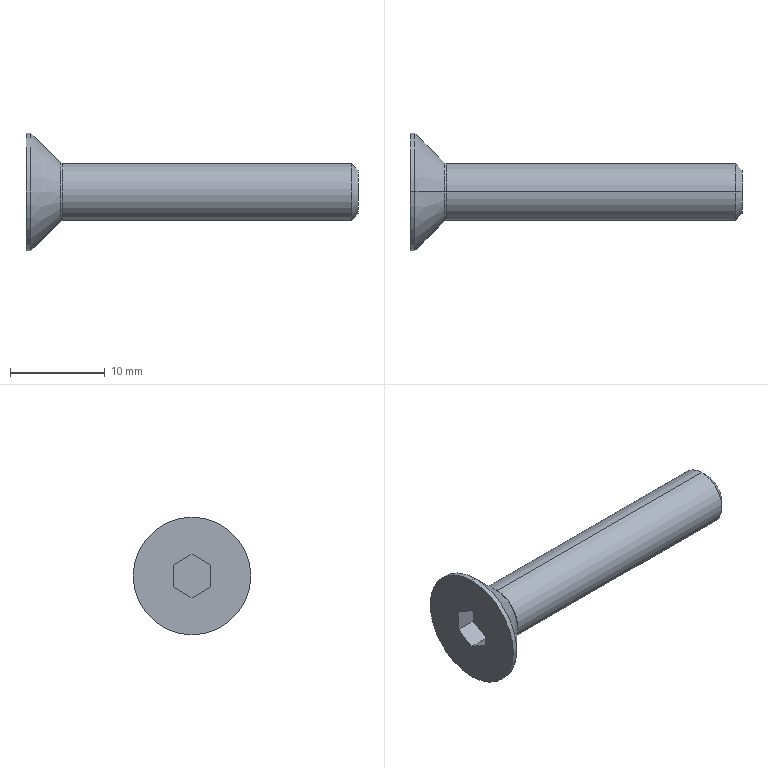Part | STEP file | 1 solid | 19 faces | box 35 x 12.399 x 12.399 mm | volume 1134 mm3 | plane 9 | cylinder 4 | cone 4 | spline 2 | commonest cylinder face diameters 6 x2 12.399 x2
STEP:
#1=CARTESIAN_POINT('',(0.,0.,0.));
#2=DIRECTION('',(0.,0.,1.));
#3=DIRECTION('',(1.,0.,0.));
#4=AXIS2_PLACEMENT_3D('',#1,#2,#3);
#5=CARTESIAN_POINT('',(-1.52,-2.,-1.155));
#6=VERTEX_POINT('',#5);
#7=CARTESIAN_POINT('',(-1.52,-2.,1.155));
#8=VERTEX_POINT('',#7);
#9=CARTESIAN_POINT('',(-1.52,-2.,-1.155));
#10=DIRECTION('',(0.,0.,1.));
#11=VECTOR('',#10,1.);
#12=LINE('',#9,#11);
#13=CARTESIAN_POINT('',(-1.52,0.,0.));
#14=DIRECTION('',(-1.,0.,0.));
#15=DIRECTION('',(0.,0.,1.));
#16=AXIS2_PLACEMENT_3D('',#13,#14,#15);
#17=PLANE('',#16);
#18=CARTESIAN_POINT('',(-1.155,-2.));
#19=DIRECTION('',(1.,0.));
#20=VECTOR('',#19,1.);
#21=LINE('',#18,#20);
#22=(GEOMETRIC_REPRESENTATION_CONTEXT(2)PARAMETRIC_REPRESENTATION_CONTEXT()REPRESENTATION_CONTEXT('',''));
#23=DEFINITIONAL_REPRESENTATION('',(#21),#22);
#24=PCURVE('',#17,#23);
#25=CARTESIAN_POINT('',(-1.52,-2.,-1.155));
#26=DIRECTION('',(0.,-1.,0.));
#27=DIRECTION('',(0.,0.,-1.));
#28=AXIS2_PLACEMENT_3D('',#25,#26,#27);
#29=PLANE('',#28);
#30=CARTESIAN_POINT('',(0.,0.));
#31=DIRECTION('',(-1.,0.));
#32=VECTOR('',#31,1.);
#33=LINE('',#30,#32);
#34=(GEOMETRIC_REPRESENTATION_CONTEXT(2)PARAMETRIC_REPRESENTATION_CONTEXT()REPRESENTATION_CONTEXT('',''));
#35=DEFINITIONAL_REPRESENTATION('',(#33),#34);
#36=PCURVE('',#29,#35);
#37=SURFACE_CURVE('',#12,(#24,#36),.PCURVE_S1.);
#38=EDGE_CURVE('',#6,#8,#37,.T.);
#39=ORIENTED_EDGE('',*,*,#38,.T.);
#40=CARTESIAN_POINT('',(-1.52,0.,2.309));
#41=VERTEX_POINT('',#40);
#42=CARTESIAN_POINT('',(-1.52,-2.,1.155));
#43=DIRECTION('',(0.,0.866,0.5));
#44=VECTOR('',#43,1.);
#45=LINE('',#42,#44);
#46=CARTESIAN_POINT('',(1.155,-2.));
#47=DIRECTION('',(0.5,0.866));
#48=VECTOR('',#47,1.);
#49=LINE('',#46,#48);
#50=(GEOMETRIC_REPRESENTATION_CONTEXT(2)PARAMETRIC_REPRESENTATION_CONTEXT()REPRESENTATION_CONTEXT('',''));
#51=DEFINITIONAL_REPRESENTATION('',(#49),#50);
#52=PCURVE('',#17,#51);
#53=CARTESIAN_POINT('',(-1.52,-2.,1.155));
#54=DIRECTION('',(0.,-0.5,0.866));
#55=DIRECTION('',(-1.,0.,0.));
#56=AXIS2_PLACEMENT_3D('',#53,#54,#55);
#57=PLANE('',#56);
#58=CARTESIAN_POINT('',(0.,0.));
#59=DIRECTION('',(0.,-1.));
#60=VECTOR('',#59,1.);
#61=LINE('',#58,#60);
#62=(GEOMETRIC_REPRESENTATION_CONTEXT(2)PARAMETRIC_REPRESENTATION_CONTEXT()REPRESENTATION_CONTEXT('',''));
#63=DEFINITIONAL_REPRESENTATION('',(#61),#62);
#64=PCURVE('',#57,#63);
#65=SURFACE_CURVE('',#45,(#52,#64),.PCURVE_S1.);
#66=EDGE_CURVE('',#8,#41,#65,.T.);
#67=ORIENTED_EDGE('',*,*,#66,.T.);
#68=CARTESIAN_POINT('',(-1.52,2.,1.155));
#69=VERTEX_POINT('',#68);
#70=CARTESIAN_POINT('',(-1.52,0.,2.309));
#71=DIRECTION('',(0.,0.866,-0.5));
#72=VECTOR('',#71,1.);
#73=LINE('',#70,#72);
#74=CARTESIAN_POINT('',(2.309,0.));
#75=DIRECTION('',(-0.5,0.866));
#76=VECTOR('',#75,1.);
#77=LINE('',#74,#76);
#78=(GEOMETRIC_REPRESENTATION_CONTEXT(2)PARAMETRIC_REPRESENTATION_CONTEXT()REPRESENTATION_CONTEXT('',''));
#79=DEFINITIONAL_REPRESENTATION('',(#77),#78);
#80=PCURVE('',#17,#79);
#81=CARTESIAN_POINT('',(-1.52,0.,2.309));
#82=DIRECTION('',(0.,0.5,0.866));
#83=DIRECTION('',(1.,0.,0.));
#84=AXIS2_PLACEMENT_3D('',#81,#82,#83);
#85=PLANE('',#84);
#86=CARTESIAN_POINT('',(0.,0.));
#87=DIRECTION('',(0.,1.));
#88=VECTOR('',#87,1.);
#89=LINE('',#86,#88);
#90=(GEOMETRIC_REPRESENTATION_CONTEXT(2)PARAMETRIC_REPRESENTATION_CONTEXT()REPRESENTATION_CONTEXT('',''));
#91=DEFINITIONAL_REPRESENTATION('',(#89),#90);
#92=PCURVE('',#85,#91);
#93=SURFACE_CURVE('',#73,(#80,#92),.PCURVE_S1.);
#94=EDGE_CURVE('',#41,#69,#93,.T.);
#95=ORIENTED_EDGE('',*,*,#94,.T.);
#96=CARTESIAN_POINT('',(-1.52,2.,-1.155));
#97=VERTEX_POINT('',#96);
#98=CARTESIAN_POINT('',(-1.52,2.,1.155));
#99=DIRECTION('',(0.,0.,-1.));
#100=VECTOR('',#99,1.);
#101=LINE('',#98,#100);
#102=CARTESIAN_POINT('',(1.155,2.));
#103=DIRECTION('',(-1.,0.));
#104=VECTOR('',#103,1.);
#105=LINE('',#102,#104);
#106=(GEOMETRIC_REPRESENTATION_CONTEXT(2)PARAMETRIC_REPRESENTATION_CONTEXT()REPRESENTATION_CONTEXT('',''));
#107=DEFINITIONAL_REPRESENTATION('',(#105),#106);
#108=PCURVE('',#17,#107);
#109=CARTESIAN_POINT('',(-1.52,2.,1.155));
#110=DIRECTION('',(0.,1.,0.));
#111=DIRECTION('',(0.,0.,-1.));
#112=AXIS2_PLACEMENT_3D('',#109,#110,#111);
#113=PLANE('',#112);
#114=CARTESIAN_POINT('',(0.,0.));
#115=DIRECTION('',(1.,0.));
#116=VECTOR('',#115,1.);
#117=LINE('',#114,#116);
#118=(GEOMETRIC_REPRESENTATION_CONTEXT(2)PARAMETRIC_REPRESENTATION_CONTEXT()REPRESENTATION_CONTEXT('',''));
#119=DEFINITIONAL_REPRESENTATION('',(#117),#118);
#120=PCURVE('',#113,#119);
#121=SURFACE_CURVE('',#101,(#108,#120),.PCURVE_S1.);
#122=EDGE_CURVE('',#69,#97,#121,.T.);
#123=ORIENTED_EDGE('',*,*,#122,.T.);
#124=CARTESIAN_POINT('',(-1.52,0.,-2.309));
#125=VERTEX_POINT('',#124);
#126=CARTESIAN_POINT('',(-1.52,2.,-1.155));
#127=DIRECTION('',(0.,-0.866,-0.5));
#128=VECTOR('',#127,1.);
#129=LINE('',#126,#128);
#130=CARTESIAN_POINT('',(-1.155,2.));
#131=DIRECTION('',(-0.5,-0.866));
#132=VECTOR('',#131,1.);
#133=LINE('',#130,#132);
#134=(GEOMETRIC_REPRESENTATION_CONTEXT(2)PARAMETRIC_REPRESENTATION_CONTEXT()REPRESENTATION_CONTEXT('',''));
#135=DEFINITIONAL_REPRESENTATION('',(#133),#134);
#136=PCURVE('',#17,#135);
#137=CARTESIAN_POINT('',(-1.52,2.,-1.155));
#138=DIRECTION('',(0.,0.5,-0.866));
#139=DIRECTION('',(-1.,0.,0.));
#140=AXIS2_PLACEMENT_3D('',#137,#138,#139);
#141=PLANE('',#140);
#142=CARTESIAN_POINT('',(0.,0.));
#143=DIRECTION('',(0.,-1.));
#144=VECTOR('',#143,1.);
#145=LINE('',#142,#144);
#146=(GEOMETRIC_REPRESENTATION_CONTEXT(2)PARAMETRIC_REPRESENTATION_CONTEXT()REPRESENTATION_CONTEXT('',''));
#147=DEFINITIONAL_REPRESENTATION('',(#145),#146);
#148=PCURVE('',#141,#147);
#149=SURFACE_CURVE('',#129,(#136,#148),.PCURVE_S1.);
#150=EDGE_CURVE('',#97,#125,#149,.T.);
#151=ORIENTED_EDGE('',*,*,#150,.T.);
#152=CARTESIAN_POINT('',(-1.52,0.,-2.309));
#153=DIRECTION('',(0.,-0.866,0.5));
#154=VECTOR('',#153,1.);
#155=LINE('',#152,#154);
#156=CARTESIAN_POINT('',(-2.309,0.));
#157=DIRECTION('',(0.5,-0.866));
#158=VECTOR('',#157,1.);
#159=LINE('',#156,#158);
#160=(GEOMETRIC_REPRESENTATION_CONTEXT(2)PARAMETRIC_REPRESENTATION_CONTEXT()REPRESENTATION_CONTEXT('',''));
#161=DEFINITIONAL_REPRESENTATION('',(#159),#160);
#162=PCURVE('',#17,#161);
#163=CARTESIAN_POINT('',(-1.52,0.,-2.309));
#164=DIRECTION('',(0.,-0.5,-0.866));
#165=DIRECTION('',(0.,-0.866,0.5));
#166=AXIS2_PLACEMENT_3D('',#163,#164,#165);
#167=PLANE('',#166);
#168=CARTESIAN_POINT('',(0.,0.));
#169=DIRECTION('',(1.,0.));
#170=VECTOR('',#169,1.);
#171=LINE('',#168,#170);
#172=(GEOMETRIC_REPRESENTATION_CONTEXT(2)PARAMETRIC_REPRESENTATION_CONTEXT()REPRESENTATION_CONTEXT('',''));
#173=DEFINITIONAL_REPRESENTATION('',(#171),#172);
#174=PCURVE('',#167,#173);
#175=SURFACE_CURVE('',#155,(#162,#174),.PCURVE_S1.);
#176=EDGE_CURVE('',#125,#6,#175,.T.);
#177=ORIENTED_EDGE('',*,*,#176,.T.);
#178=EDGE_LOOP('',(#39,#67,#95,#123,#151,#177));
#179=FACE_BOUND('',#178,.T.);
#180=ADVANCED_FACE('',(#179),#17,.T.);
#181=CARTESIAN_POINT('',(-3.72,0.,-2.309));
#182=VERTEX_POINT('',#181);
#183=CARTESIAN_POINT('',(-1.52,0.,-2.309));
#184=DIRECTION('',(1.,0.,0.));
#185=VECTOR('',#184,1.);
#186=LINE('',#183,#185);
#187=CARTESIAN_POINT('',(0.,-2.309));
#188=DIRECTION('',(-1.,0.));
#189=VECTOR('',#188,1.);
#190=LINE('',#187,#189);
#191=(GEOMETRIC_REPRESENTATION_CONTEXT(2)PARAMETRIC_REPRESENTATION_CONTEXT()REPRESENTATION_CONTEXT('',''));
#192=DEFINITIONAL_REPRESENTATION('',(#190),#191);
#193=PCURVE('',#141,#192);
#194=CARTESIAN_POINT('',(0.,0.));
#195=DIRECTION('',(0.,-1.));
#196=VECTOR('',#195,1.);
#197=LINE('',#194,#196);
#198=(GEOMETRIC_REPRESENTATION_CONTEXT(2)PARAMETRIC_REPRESENTATION_CONTEXT()REPRESENTATION_CONTEXT('',''));
#199=DEFINITIONAL_REPRESENTATION('',(#197),#198);
#200=PCURVE('',#167,#199);
#201=SURFACE_CURVE('',#186,(#193,#200),.PCURVE_S1.);
#202=EDGE_CURVE('',#182,#125,#201,.T.);
#203=ORIENTED_EDGE('',*,*,#202,.T.);
#204=ORIENTED_EDGE('',*,*,#150,.F.);
#205=CARTESIAN_POINT('',(-3.72,2.,-1.155));
#206=VERTEX_POINT('',#205);
#207=CARTESIAN_POINT('',(-1.52,2.,-1.155));
#208=DIRECTION('',(-1.,0.,0.));
#209=VECTOR('',#208,1.);
#210=LINE('',#207,#209);
#211=CARTESIAN_POINT('',(0.,0.));
#212=DIRECTION('',(1.,0.));
#213=VECTOR('',#212,1.);
#214=LINE('',#211,#213);
#215=(GEOMETRIC_REPRESENTATION_CONTEXT(2)PARAMETRIC_REPRESENTATION_CONTEXT()REPRESENTATION_CONTEXT('',''));
#216=DEFINITIONAL_REPRESENTATION('',(#214),#215);
#217=PCURVE('',#141,#216);
#218=CARTESIAN_POINT('',(2.309,0.));
#219=DIRECTION('',(0.,1.));
#220=VECTOR('',#219,1.);
#221=LINE('',#218,#220);
#222=(GEOMETRIC_REPRESENTATION_CONTEXT(2)PARAMETRIC_REPRESENTATION_CONTEXT()REPRESENTATION_CONTEXT('',''));
#223=DEFINITIONAL_REPRESENTATION('',(#221),#222);
#224=PCURVE('',#113,#223);
#225=SURFACE_CURVE('',#210,(#217,#224),.PCURVE_S1.);
#226=EDGE_CURVE('',#97,#206,#225,.T.);
#227=ORIENTED_EDGE('',*,*,#226,.T.);
#228=CARTESIAN_POINT('',(-3.72,2.,-1.155));
#229=DIRECTION('',(0.,-0.866,-0.5));
#230=VECTOR('',#229,1.);
#231=LINE('',#228,#230);
#232=CARTESIAN_POINT('',(2.2,0.));
#233=DIRECTION('',(0.,-1.));
#234=VECTOR('',#233,1.);
#235=LINE('',#232,#234);
#236=(GEOMETRIC_REPRESENTATION_CONTEXT(2)PARAMETRIC_REPRESENTATION_CONTEXT()REPRESENTATION_CONTEXT('',''));
#237=DEFINITIONAL_REPRESENTATION('',(#235),#236);
#238=PCURVE('',#141,#237);
#239=CARTESIAN_POINT('',(-3.72,6.2,0.));
#240=DIRECTION('',(1.,0.,0.));
#241=DIRECTION('',(0.,1.,0.));
#242=AXIS2_PLACEMENT_3D('',#239,#240,#241);
#243=PLANE('',#242);
#244=CARTESIAN_POINT('',(-4.2,-1.155));
#245=DIRECTION('',(-0.866,-0.5));
#246=VECTOR('',#245,1.);
#247=LINE('',#244,#246);
#248=(GEOMETRIC_REPRESENTATION_CONTEXT(2)PARAMETRIC_REPRESENTATION_CONTEXT()REPRESENTATION_CONTEXT('',''));
#249=DEFINITIONAL_REPRESENTATION('',(#247),#248);
#250=PCURVE('',#243,#249);
#251=SURFACE_CURVE('',#231,(#238,#250),.PCURVE_S1.);
#252=EDGE_CURVE('',#206,#182,#251,.T.);
#253=ORIENTED_EDGE('',*,*,#252,.T.);
#254=EDGE_LOOP('',(#203,#204,#227,#253));
#255=FACE_BOUND('',#254,.T.);
#256=ADVANCED_FACE('',(#255),#141,.F.);
#257=CARTESIAN_POINT('',(-3.72,-2.,-1.155));
#258=VERTEX_POINT('',#257);
#259=CARTESIAN_POINT('',(-1.52,-2.,-1.155));
#260=DIRECTION('',(1.,0.,0.));
#261=VECTOR('',#260,1.);
#262=LINE('',#259,#261);
#263=CARTESIAN_POINT('',(2.309,0.));
#264=DIRECTION('',(0.,-1.));
#265=VECTOR('',#264,1.);
#266=LINE('',#263,#265);
#267=(GEOMETRIC_REPRESENTATION_CONTEXT(2)PARAMETRIC_REPRESENTATION_CONTEXT()REPRESENTATION_CONTEXT('',''));
#268=DEFINITIONAL_REPRESENTATION('',(#266),#267);
#269=PCURVE('',#167,#268);
#270=CARTESIAN_POINT('',(0.,0.));
#271=DIRECTION('',(0.,1.));
#272=VECTOR('',#271,1.);
#273=LINE('',#270,#272);
#274=(GEOMETRIC_REPRESENTATION_CONTEXT(2)PARAMETRIC_REPRESENTATION_CONTEXT()REPRESENTATION_CONTEXT('',''));
#275=DEFINITIONAL_REPRESENTATION('',(#273),#274);
#276=PCURVE('',#29,#275);
#277=SURFACE_CURVE('',#262,(#269,#276),.PCURVE_S1.);
#278=EDGE_CURVE('',#258,#6,#277,.T.);
#279=ORIENTED_EDGE('',*,*,#278,.T.);
#280=ORIENTED_EDGE('',*,*,#176,.F.);
#281=ORIENTED_EDGE('',*,*,#202,.F.);
#282=CARTESIAN_POINT('',(-3.72,0.,-2.309));
#283=DIRECTION('',(0.,-0.866,0.5));
#284=VECTOR('',#283,1.);
#285=LINE('',#282,#284);
#286=CARTESIAN_POINT('',(0.,2.2));
#287=DIRECTION('',(1.,0.));
#288=VECTOR('',#287,1.);
#289=LINE('',#286,#288);
#290=(GEOMETRIC_REPRESENTATION_CONTEXT(2)PARAMETRIC_REPRESENTATION_CONTEXT()REPRESENTATION_CONTEXT('',''));
#291=DEFINITIONAL_REPRESENTATION('',(#289),#290);
#292=PCURVE('',#167,#291);
#293=CARTESIAN_POINT('',(-6.2,-2.309));
#294=DIRECTION('',(-0.866,0.5));
#295=VECTOR('',#294,1.);
#296=LINE('',#293,#295);
#297=(GEOMETRIC_REPRESENTATION_CONTEXT(2)PARAMETRIC_REPRESENTATION_CONTEXT()REPRESENTATION_CONTEXT('',''));
#298=DEFINITIONAL_REPRESENTATION('',(#296),#297);
#299=PCURVE('',#243,#298);
#300=SURFACE_CURVE('',#285,(#292,#299),.PCURVE_S1.);
#301=EDGE_CURVE('',#182,#258,#300,.T.);
#302=ORIENTED_EDGE('',*,*,#301,.T.);
#303=EDGE_LOOP('',(#279,#280,#281,#302));
#304=FACE_BOUND('',#303,.T.);
#305=ADVANCED_FACE('',(#304),#167,.F.);
#306=CARTESIAN_POINT('',(-3.72,-2.,1.155));
#307=VERTEX_POINT('',#306);
#308=CARTESIAN_POINT('',(-1.52,-2.,1.155));
#309=DIRECTION('',(1.,0.,0.));
#310=VECTOR('',#309,1.);
#311=LINE('',#308,#310);
#312=CARTESIAN_POINT('',(-2.309,0.));
#313=DIRECTION('',(0.,1.));
#314=VECTOR('',#313,1.);
#315=LINE('',#312,#314);
#316=(GEOMETRIC_REPRESENTATION_CONTEXT(2)PARAMETRIC_REPRESENTATION_CONTEXT()REPRESENTATION_CONTEXT('',''));
#317=DEFINITIONAL_REPRESENTATION('',(#315),#316);
#318=PCURVE('',#29,#317);
#319=CARTESIAN_POINT('',(0.,0.));
#320=DIRECTION('',(-1.,0.));
#321=VECTOR('',#320,1.);
#322=LINE('',#319,#321);
#323=(GEOMETRIC_REPRESENTATION_CONTEXT(2)PARAMETRIC_REPRESENTATION_CONTEXT()REPRESENTATION_CONTEXT('',''));
#324=DEFINITIONAL_REPRESENTATION('',(#322),#323);
#325=PCURVE('',#57,#324);
#326=SURFACE_CURVE('',#311,(#318,#325),.PCURVE_S1.);
#327=EDGE_CURVE('',#307,#8,#326,.T.);
#328=ORIENTED_EDGE('',*,*,#327,.T.);
#329=ORIENTED_EDGE('',*,*,#38,.F.);
#330=ORIENTED_EDGE('',*,*,#278,.F.);
#331=CARTESIAN_POINT('',(-3.72,-2.,0.));
#332=DIRECTION('',(0.,0.,1.));
#333=VECTOR('',#332,1.);
#334=LINE('',#331,#333);
#335=CARTESIAN_POINT('',(-1.155,-2.2));
#336=DIRECTION('',(-1.,0.));
#337=VECTOR('',#336,1.);
#338=LINE('',#335,#337);
#339=(GEOMETRIC_REPRESENTATION_CONTEXT(2)PARAMETRIC_REPRESENTATION_CONTEXT()REPRESENTATION_CONTEXT('',''));
#340=DEFINITIONAL_REPRESENTATION('',(#338),#339);
#341=PCURVE('',#29,#340);
#342=CARTESIAN_POINT('',(-8.2,0.));
#343=DIRECTION('',(0.,1.));
#344=VECTOR('',#343,1.);
#345=LINE('',#342,#344);
#346=(GEOMETRIC_REPRESENTATION_CONTEXT(2)PARAMETRIC_REPRESENTATION_CONTEXT()REPRESENTATION_CONTEXT('',''));
#347=DEFINITIONAL_REPRESENTATION('',(#345),#346);
#348=PCURVE('',#243,#347);
#349=SURFACE_CURVE('',#334,(#341,#348),.PCURVE_S1.);
#350=EDGE_CURVE('',#258,#307,#349,.T.);
#351=ORIENTED_EDGE('',*,*,#350,.T.);
#352=EDGE_LOOP('',(#328,#329,#330,#351));
#353=FACE_BOUND('',#352,.T.);
#354=ADVANCED_FACE('',(#353),#29,.F.);
#355=CARTESIAN_POINT('',(-3.72,0.,2.309));
#356=VERTEX_POINT('',#355);
#357=CARTESIAN_POINT('',(-1.52,0.,2.309));
#358=DIRECTION('',(1.,0.,0.));
#359=VECTOR('',#358,1.);
#360=LINE('',#357,#359);
#361=CARTESIAN_POINT('',(0.,-2.309));
#362=DIRECTION('',(-1.,0.));
#363=VECTOR('',#362,1.);
#364=LINE('',#361,#363);
#365=(GEOMETRIC_REPRESENTATION_CONTEXT(2)PARAMETRIC_REPRESENTATION_CONTEXT()REPRESENTATION_CONTEXT('',''));
#366=DEFINITIONAL_REPRESENTATION('',(#364),#365);
#367=PCURVE('',#57,#366);
#368=CARTESIAN_POINT('',(0.,0.));
#369=DIRECTION('',(1.,0.));
#370=VECTOR('',#369,1.);
#371=LINE('',#368,#370);
#372=(GEOMETRIC_REPRESENTATION_CONTEXT(2)PARAMETRIC_REPRESENTATION_CONTEXT()REPRESENTATION_CONTEXT('',''));
#373=DEFINITIONAL_REPRESENTATION('',(#371),#372);
#374=PCURVE('',#85,#373);
#375=SURFACE_CURVE('',#360,(#367,#374),.PCURVE_S1.);
#376=EDGE_CURVE('',#356,#41,#375,.T.);
#377=ORIENTED_EDGE('',*,*,#376,.T.);
#378=ORIENTED_EDGE('',*,*,#66,.F.);
#379=ORIENTED_EDGE('',*,*,#327,.F.);
#380=CARTESIAN_POINT('',(-3.72,-2.,1.155));
#381=DIRECTION('',(0.,0.866,0.5));
#382=VECTOR('',#381,1.);
#383=LINE('',#380,#382);
#384=CARTESIAN_POINT('',(2.2,0.));
#385=DIRECTION('',(0.,-1.));
#386=VECTOR('',#385,1.);
#387=LINE('',#384,#386);
#388=(GEOMETRIC_REPRESENTATION_CONTEXT(2)PARAMETRIC_REPRESENTATION_CONTEXT()REPRESENTATION_CONTEXT('',''));
#389=DEFINITIONAL_REPRESENTATION('',(#387),#388);
#390=PCURVE('',#57,#389);
#391=CARTESIAN_POINT('',(-8.2,1.155));
#392=DIRECTION('',(0.866,0.5));
#393=VECTOR('',#392,1.);
#394=LINE('',#391,#393);
#395=(GEOMETRIC_REPRESENTATION_CONTEXT(2)PARAMETRIC_REPRESENTATION_CONTEXT()REPRESENTATION_CONTEXT('',''));
#396=DEFINITIONAL_REPRESENTATION('',(#394),#395);
#397=PCURVE('',#243,#396);
#398=SURFACE_CURVE('',#383,(#390,#397),.PCURVE_S1.);
#399=EDGE_CURVE('',#307,#356,#398,.T.);
#400=ORIENTED_EDGE('',*,*,#399,.T.);
#401=EDGE_LOOP('',(#377,#378,#379,#400));
#402=FACE_BOUND('',#401,.T.);
#403=ADVANCED_FACE('',(#402),#57,.F.);
#404=CARTESIAN_POINT('',(-3.72,2.,1.155));
#405=VERTEX_POINT('',#404);
#406=CARTESIAN_POINT('',(-1.52,2.,1.155));
#407=DIRECTION('',(1.,0.,0.));
#408=VECTOR('',#407,1.);
#409=LINE('',#406,#408);
#410=CARTESIAN_POINT('',(0.,2.309));
#411=DIRECTION('',(1.,0.));
#412=VECTOR('',#411,1.);
#413=LINE('',#410,#412);
#414=(GEOMETRIC_REPRESENTATION_CONTEXT(2)PARAMETRIC_REPRESENTATION_CONTEXT()REPRESENTATION_CONTEXT('',''));
#415=DEFINITIONAL_REPRESENTATION('',(#413),#414);
#416=PCURVE('',#85,#415);
#417=CARTESIAN_POINT('',(0.,0.));
#418=DIRECTION('',(0.,-1.));
#419=VECTOR('',#418,1.);
#420=LINE('',#417,#419);
#421=(GEOMETRIC_REPRESENTATION_CONTEXT(2)PARAMETRIC_REPRESENTATION_CONTEXT()REPRESENTATION_CONTEXT('',''));
#422=DEFINITIONAL_REPRESENTATION('',(#420),#421);
#423=PCURVE('',#113,#422);
#424=SURFACE_CURVE('',#409,(#416,#423),.PCURVE_S1.);
#425=EDGE_CURVE('',#405,#69,#424,.T.);
#426=ORIENTED_EDGE('',*,*,#425,.T.);
#427=ORIENTED_EDGE('',*,*,#94,.F.);
#428=ORIENTED_EDGE('',*,*,#376,.F.);
#429=CARTESIAN_POINT('',(-3.72,0.,2.309));
#430=DIRECTION('',(0.,0.866,-0.5));
#431=VECTOR('',#430,1.);
#432=LINE('',#429,#431);
#433=CARTESIAN_POINT('',(-2.2,0.));
#434=DIRECTION('',(0.,1.));
#435=VECTOR('',#434,1.);
#436=LINE('',#433,#435);
#437=(GEOMETRIC_REPRESENTATION_CONTEXT(2)PARAMETRIC_REPRESENTATION_CONTEXT()REPRESENTATION_CONTEXT('',''));
#438=DEFINITIONAL_REPRESENTATION('',(#436),#437);
#439=PCURVE('',#85,#438);
#440=CARTESIAN_POINT('',(-6.2,2.309));
#441=DIRECTION('',(0.866,-0.5));
#442=VECTOR('',#441,1.);
#443=LINE('',#440,#442);
#444=(GEOMETRIC_REPRESENTATION_CONTEXT(2)PARAMETRIC_REPRESENTATION_CONTEXT()REPRESENTATION_CONTEXT('',''));
#445=DEFINITIONAL_REPRESENTATION('',(#443),#444);
#446=PCURVE('',#243,#445);
#447=SURFACE_CURVE('',#432,(#439,#446),.PCURVE_S1.);
#448=EDGE_CURVE('',#356,#405,#447,.T.);
#449=ORIENTED_EDGE('',*,*,#448,.T.);
#450=EDGE_LOOP('',(#426,#427,#428,#449));
#451=FACE_BOUND('',#450,.T.);
#452=ADVANCED_FACE('',(#451),#85,.F.);
#453=ORIENTED_EDGE('',*,*,#226,.F.);
#454=ORIENTED_EDGE('',*,*,#122,.F.);
#455=ORIENTED_EDGE('',*,*,#425,.F.);
#456=CARTESIAN_POINT('',(-3.72,2.,0.));
#457=DIRECTION('',(0.,0.,-1.));
#458=VECTOR('',#457,1.);
#459=LINE('',#456,#458);
#460=CARTESIAN_POINT('',(1.155,2.2));
#461=DIRECTION('',(1.,0.));
#462=VECTOR('',#461,1.);
#463=LINE('',#460,#462);
#464=(GEOMETRIC_REPRESENTATION_CONTEXT(2)PARAMETRIC_REPRESENTATION_CONTEXT()REPRESENTATION_CONTEXT('',''));
#465=DEFINITIONAL_REPRESENTATION('',(#463),#464);
#466=PCURVE('',#113,#465);
#467=CARTESIAN_POINT('',(-4.2,0.));
#468=DIRECTION('',(0.,-1.));
#469=VECTOR('',#468,1.);
#470=LINE('',#467,#469);
#471=(GEOMETRIC_REPRESENTATION_CONTEXT(2)PARAMETRIC_REPRESENTATION_CONTEXT()REPRESENTATION_CONTEXT('',''));
#472=DEFINITIONAL_REPRESENTATION('',(#470),#471);
#473=PCURVE('',#243,#472);
#474=SURFACE_CURVE('',#459,(#466,#473),.PCURVE_S1.);
#475=EDGE_CURVE('',#405,#206,#474,.T.);
#476=ORIENTED_EDGE('',*,*,#475,.T.);
#477=EDGE_LOOP('',(#453,#454,#455,#476));
#478=FACE_BOUND('',#477,.T.);
#479=ADVANCED_FACE('',(#478),#113,.F.);
#480=ORIENTED_EDGE('',*,*,#448,.F.);
#481=ORIENTED_EDGE('',*,*,#399,.F.);
#482=ORIENTED_EDGE('',*,*,#350,.F.);
#483=ORIENTED_EDGE('',*,*,#301,.F.);
#484=ORIENTED_EDGE('',*,*,#252,.F.);
#485=ORIENTED_EDGE('',*,*,#475,.F.);
#486=EDGE_LOOP('',(#480,#481,#482,#483,#484,#485));
#487=FACE_BOUND('',#486,.T.);
#488=CARTESIAN_POINT('',(-3.72,0.,6.2));
#489=VERTEX_POINT('',#488);
#490=CARTESIAN_POINT('',(-3.72,0.,-6.2));
#491=VERTEX_POINT('',#490);
#492=CARTESIAN_POINT('',(-3.72,0.,0.));
#493=DIRECTION('',(1.,0.,0.));
#494=DIRECTION('',(0.,0.,1.));
#495=AXIS2_PLACEMENT_3D('',#492,#493,#494);
#496=CIRCLE('',#495,6.2);
#497=CARTESIAN_POINT('',(-6.2,0.));
#498=DIRECTION('',(0.,1.));
#499=AXIS2_PLACEMENT_2D('',#497,#498);
#500=CIRCLE('',#499,6.2);
#501=(GEOMETRIC_REPRESENTATION_CONTEXT(2)PARAMETRIC_REPRESENTATION_CONTEXT()REPRESENTATION_CONTEXT('',''));
#502=DEFINITIONAL_REPRESENTATION('',(#500),#501);
#503=PCURVE('',#243,#502);
#504=CARTESIAN_POINT('',(-30.898,0.,0.));
#505=DIRECTION('',(-1.,0.,0.));
#506=DIRECTION('',(0.,0.,1.));
#507=AXIS2_PLACEMENT_3D('',#504,#505,#506);
#508=CYLINDRICAL_SURFACE('',#507,6.2);
#509=CARTESIAN_POINT('',(6.283,-27.178));
#510=DIRECTION('',(-1.,0.));
#511=VECTOR('',#510,1.);
#512=LINE('',#509,#511);
#513=(GEOMETRIC_REPRESENTATION_CONTEXT(2)PARAMETRIC_REPRESENTATION_CONTEXT()REPRESENTATION_CONTEXT('',''));
#514=DEFINITIONAL_REPRESENTATION('',(#512),#513);
#515=PCURVE('',#508,#514);
#516=SURFACE_CURVE('',#496,(#503,#515),.PCURVE_S1.);
#517=EDGE_CURVE('',#489,#491,#516,.T.);
#518=ORIENTED_EDGE('',*,*,#517,.F.);
#519=CARTESIAN_POINT('',(-3.72,0.,0.));
#520=DIRECTION('',(1.,0.,0.));
#521=DIRECTION('',(0.,0.,1.));
#522=AXIS2_PLACEMENT_3D('',#519,#520,#521);
#523=CIRCLE('',#522,6.2);
#524=CARTESIAN_POINT('',(-6.2,0.));
#525=DIRECTION('',(0.,1.));
#526=AXIS2_PLACEMENT_2D('',#524,#525);
#527=CIRCLE('',#526,6.2);
#528=(GEOMETRIC_REPRESENTATION_CONTEXT(2)PARAMETRIC_REPRESENTATION_CONTEXT()REPRESENTATION_CONTEXT('',''));
#529=DEFINITIONAL_REPRESENTATION('',(#527),#528);
#530=PCURVE('',#243,#529);
#531=CARTESIAN_POINT('',(-30.898,0.,0.));
#532=DIRECTION('',(-1.,0.,0.));
#533=DIRECTION('',(0.,0.,1.));
#534=AXIS2_PLACEMENT_3D('',#531,#532,#533);
#535=CYLINDRICAL_SURFACE('',#534,6.2);
#536=CARTESIAN_POINT('',(6.283,-27.178));
#537=DIRECTION('',(-1.,0.));
#538=VECTOR('',#537,1.);
#539=LINE('',#536,#538);
#540=(GEOMETRIC_REPRESENTATION_CONTEXT(2)PARAMETRIC_REPRESENTATION_CONTEXT()REPRESENTATION_CONTEXT('',''));
#541=DEFINITIONAL_REPRESENTATION('',(#539),#540);
#542=PCURVE('',#535,#541);
#543=SURFACE_CURVE('',#523,(#530,#542),.PCURVE_S1.);
#544=EDGE_CURVE('',#491,#489,#543,.T.);
#545=ORIENTED_EDGE('',*,*,#544,.F.);
#546=EDGE_LOOP('',(#518,#545));
#547=FACE_BOUND('',#546,.T.);
#548=ADVANCED_FACE('',(#487,#547),#243,.F.);
#549=CARTESIAN_POINT('',(-3.2,0.,-6.2));
#550=VERTEX_POINT('',#549);
#551=CARTESIAN_POINT('',(-30.898,0.,-6.2));
#552=DIRECTION('',(-1.,0.,0.));
#553=VECTOR('',#552,1.);
#554=LINE('',#551,#553);
#555=CARTESIAN_POINT('',(3.142,0.));
#556=DIRECTION('',(0.,1.));
#557=VECTOR('',#556,1.);
#558=LINE('',#555,#557);
#559=(GEOMETRIC_REPRESENTATION_CONTEXT(2)PARAMETRIC_REPRESENTATION_CONTEXT()REPRESENTATION_CONTEXT('',''));
#560=DEFINITIONAL_REPRESENTATION('',(#558),#559);
#561=PCURVE('',#508,#560);
#562=CARTESIAN_POINT('',(3.142,0.));
#563=DIRECTION('',(0.,1.));
#564=VECTOR('',#563,1.);
#565=LINE('',#562,#564);
#566=(GEOMETRIC_REPRESENTATION_CONTEXT(2)PARAMETRIC_REPRESENTATION_CONTEXT()REPRESENTATION_CONTEXT('',''));
#567=DEFINITIONAL_REPRESENTATION('',(#565),#566);
#568=PCURVE('',#535,#567);
#569=SURFACE_CURVE('',#554,(#561,#568),.PCURVE_S1.);
#570=EDGE_CURVE('',#550,#491,#569,.T.);
#571=ORIENTED_EDGE('',*,*,#570,.F.);
#572=CARTESIAN_POINT('',(-3.2,0.,6.2));
#573=VERTEX_POINT('',#572);
#574=CARTESIAN_POINT('',(-3.2,0.,0.));
#575=DIRECTION('',(1.,0.,0.));
#576=DIRECTION('',(0.,0.,1.));
#577=AXIS2_PLACEMENT_3D('',#574,#575,#576);
#578=CIRCLE('',#577,6.2);
#579=CARTESIAN_POINT('',(6.283,-27.698));
#580=DIRECTION('',(-1.,0.));
#581=VECTOR('',#580,1.);
#582=LINE('',#579,#581);
#583=(GEOMETRIC_REPRESENTATION_CONTEXT(2)PARAMETRIC_REPRESENTATION_CONTEXT()REPRESENTATION_CONTEXT('',''));
#584=DEFINITIONAL_REPRESENTATION('',(#582),#583);
#585=PCURVE('',#508,#584);
#586=CARTESIAN_POINT('',(-3.2,0.,0.));
#587=DIRECTION('',(-1.,0.,0.));
#588=DIRECTION('',(0.,0.,1.));
#589=AXIS2_PLACEMENT_3D('',#586,#587,#588);
#590=CONICAL_SURFACE('',#589,6.2,0.7854);
#591=CARTESIAN_POINT('',(6.283,0.));
#592=DIRECTION('',(-1.,0.));
#593=VECTOR('',#592,1.);
#594=LINE('',#591,#593);
#595=(GEOMETRIC_REPRESENTATION_CONTEXT(2)PARAMETRIC_REPRESENTATION_CONTEXT()REPRESENTATION_CONTEXT('',''));
#596=DEFINITIONAL_REPRESENTATION('',(#594),#595);
#597=PCURVE('',#590,#596);
#598=SURFACE_CURVE('',#578,(#585,#597),.PCURVE_S1.);
#599=EDGE_CURVE('',#573,#550,#598,.T.);
#600=ORIENTED_EDGE('',*,*,#599,.F.);
#601=CARTESIAN_POINT('',(-30.898,0.,6.2));
#602=DIRECTION('',(-1.,0.,0.));
#603=VECTOR('',#602,1.);
#604=LINE('',#601,#603);
#605=CARTESIAN_POINT('',(6.283,0.));
#606=DIRECTION('',(0.,1.));
#607=VECTOR('',#606,1.);
#608=LINE('',#605,#607);
#609=(GEOMETRIC_REPRESENTATION_CONTEXT(2)PARAMETRIC_REPRESENTATION_CONTEXT()REPRESENTATION_CONTEXT('',''));
#610=DEFINITIONAL_REPRESENTATION('',(#608),#609);
#611=PCURVE('',#508,#610);
#612=CARTESIAN_POINT('',(0.,0.));
#613=DIRECTION('',(0.,1.));
#614=VECTOR('',#613,1.);
#615=LINE('',#612,#614);
#616=(GEOMETRIC_REPRESENTATION_CONTEXT(2)PARAMETRIC_REPRESENTATION_CONTEXT()REPRESENTATION_CONTEXT('',''));
#617=DEFINITIONAL_REPRESENTATION('',(#615),#616);
#618=PCURVE('',#535,#617);
#619=SURFACE_CURVE('',#604,(#611,#618),.PCURVE_S1.);
#620=EDGE_CURVE('',#573,#489,#619,.T.);
#621=ORIENTED_EDGE('',*,*,#620,.T.);
#622=ORIENTED_EDGE('',*,*,#517,.T.);
#623=EDGE_LOOP('',(#571,#600,#621,#622));
#624=FACE_BOUND('',#623,.T.);
#625=ADVANCED_FACE('',(#624),#508,.T.);
#626=CARTESIAN_POINT('',(31.28,0.,2.3));
#627=VERTEX_POINT('',#626);
#628=CARTESIAN_POINT('',(31.28,0.,-2.3));
#629=VERTEX_POINT('',#628);
#630=CARTESIAN_POINT('',(31.28,0.,0.));
#631=DIRECTION('',(-1.,0.,0.));
#632=DIRECTION('',(0.,0.,1.));
#633=AXIS2_PLACEMENT_3D('',#630,#631,#632);
#634=CIRCLE('',#633,2.3);
#635=CARTESIAN_POINT('',(31.28,3.,0.));
#636=DIRECTION('',(-1.,0.,0.));
#637=DIRECTION('',(0.,0.,1.));
#638=AXIS2_PLACEMENT_3D('',#635,#636,#637);
#639=PLANE('',#638);
#640=CARTESIAN_POINT('',(0.,-3.));
#641=DIRECTION('',(1.,0.));
#642=AXIS2_PLACEMENT_2D('',#640,#641);
#643=CIRCLE('',#642,2.3);
#644=(GEOMETRIC_REPRESENTATION_CONTEXT(2)PARAMETRIC_REPRESENTATION_CONTEXT()REPRESENTATION_CONTEXT('',''));
#645=DEFINITIONAL_REPRESENTATION('',(#643),#644);
#646=PCURVE('',#639,#645);
#647=CARTESIAN_POINT('',(30.58,0.,0.));
#648=DIRECTION('',(-1.,0.,0.));
#649=DIRECTION('',(0.,0.,1.));
#650=AXIS2_PLACEMENT_3D('',#647,#648,#649);
#651=CONICAL_SURFACE('',#650,3.,0.7854);
#652=CARTESIAN_POINT('',(0.,-0.7));
#653=DIRECTION('',(1.,0.));
#654=VECTOR('',#653,1.);
#655=LINE('',#652,#654);
#656=(GEOMETRIC_REPRESENTATION_CONTEXT(2)PARAMETRIC_REPRESENTATION_CONTEXT()REPRESENTATION_CONTEXT('',''));
#657=DEFINITIONAL_REPRESENTATION('',(#655),#656);
#658=PCURVE('',#651,#657);
#659=SURFACE_CURVE('',#634,(#646,#658),.PCURVE_S1.);
#660=EDGE_CURVE('',#627,#629,#659,.T.);
#661=ORIENTED_EDGE('',*,*,#660,.F.);
#662=CARTESIAN_POINT('',(31.28,0.,0.));
#663=DIRECTION('',(-1.,0.,0.));
#664=DIRECTION('',(0.,0.,1.));
#665=AXIS2_PLACEMENT_3D('',#662,#663,#664);
#666=CIRCLE('',#665,2.3);
#667=CARTESIAN_POINT('',(0.,-3.));
#668=DIRECTION('',(1.,0.));
#669=AXIS2_PLACEMENT_2D('',#667,#668);
#670=CIRCLE('',#669,2.3);
#671=(GEOMETRIC_REPRESENTATION_CONTEXT(2)PARAMETRIC_REPRESENTATION_CONTEXT()REPRESENTATION_CONTEXT('',''));
#672=DEFINITIONAL_REPRESENTATION('',(#670),#671);
#673=PCURVE('',#639,#672);
#674=CARTESIAN_POINT('',(30.58,0.,0.));
#675=DIRECTION('',(-1.,0.,0.));
#676=DIRECTION('',(0.,0.,1.));
#677=AXIS2_PLACEMENT_3D('',#674,#675,#676);
#678=CONICAL_SURFACE('',#677,3.,0.7854);
#679=CARTESIAN_POINT('',(0.,-0.7));
#680=DIRECTION('',(1.,0.));
#681=VECTOR('',#680,1.);
#682=LINE('',#679,#681);
#683=(GEOMETRIC_REPRESENTATION_CONTEXT(2)PARAMETRIC_REPRESENTATION_CONTEXT()REPRESENTATION_CONTEXT('',''));
#684=DEFINITIONAL_REPRESENTATION('',(#682),#683);
#685=PCURVE('',#678,#684);
#686=SURFACE_CURVE('',#666,(#673,#685),.PCURVE_S1.);
#687=EDGE_CURVE('',#629,#627,#686,.T.);
#688=ORIENTED_EDGE('',*,*,#687,.F.);
#689=EDGE_LOOP('',(#661,#688));
#690=FACE_BOUND('',#689,.T.);
#691=ADVANCED_FACE('',(#690),#639,.F.);
#692=CARTESIAN_POINT('',(-0.07322,0.,-3.073));
#693=VERTEX_POINT('',#692);
#694=CARTESIAN_POINT('',(-3.2,0.,-6.2));
#695=DIRECTION('',(-0.7071,0.,-0.7071));
#696=VECTOR('',#695,1.);
#697=LINE('',#694,#696);
#698=CARTESIAN_POINT('',(3.142,0.));
#699=DIRECTION('',(0.,1.));
#700=VECTOR('',#699,1.);
#701=LINE('',#698,#700);
#702=(GEOMETRIC_REPRESENTATION_CONTEXT(2)PARAMETRIC_REPRESENTATION_CONTEXT()REPRESENTATION_CONTEXT('',''));
#703=DEFINITIONAL_REPRESENTATION('',(#701),#702);
#704=PCURVE('',#590,#703);
#705=CARTESIAN_POINT('',(-3.2,0.,0.));
#706=DIRECTION('',(-1.,0.,0.));
#707=DIRECTION('',(0.,0.,1.));
#708=AXIS2_PLACEMENT_3D('',#705,#706,#707);
#709=CONICAL_SURFACE('',#708,6.2,0.7854);
#710=CARTESIAN_POINT('',(3.142,0.));
#711=DIRECTION('',(0.,1.));
#712=VECTOR('',#711,1.);
#713=LINE('',#710,#712);
#714=(GEOMETRIC_REPRESENTATION_CONTEXT(2)PARAMETRIC_REPRESENTATION_CONTEXT()REPRESENTATION_CONTEXT('',''));
#715=DEFINITIONAL_REPRESENTATION('',(#713),#714);
#716=PCURVE('',#709,#715);
#717=SURFACE_CURVE('',#697,(#704,#716),.PCURVE_S1.);
#718=EDGE_CURVE('',#693,#550,#717,.T.);
#719=ORIENTED_EDGE('',*,*,#718,.F.);
#720=CARTESIAN_POINT('',(-0.07322,0.,3.073));
#721=VERTEX_POINT('',#720);
#722=CARTESIAN_POINT('',(-0.07322,0.,0.));
#723=DIRECTION('',(-1.,0.,0.));
#724=DIRECTION('',(0.,0.,1.));
#725=AXIS2_PLACEMENT_3D('',#722,#723,#724);
#726=CIRCLE('',#725,3.073);
#727=CARTESIAN_POINT('',(0.,-3.126));
#728=DIRECTION('',(1.,0.));
#729=VECTOR('',#728,1.);
#730=LINE('',#727,#729);
#731=(GEOMETRIC_REPRESENTATION_CONTEXT(2)PARAMETRIC_REPRESENTATION_CONTEXT()REPRESENTATION_CONTEXT('',''));
#732=DEFINITIONAL_REPRESENTATION('',(#730),#731);
#733=PCURVE('',#590,#732);
#734=CARTESIAN_POINT('',(0.1036,0.,-3.));
#735=CARTESIAN_POINT('',(0.1036,-6.,-3.));
#736=CARTESIAN_POINT('',(0.1036,-6.,3.));
#737=CARTESIAN_POINT('',(0.1036,0.,3.));
#738=CARTESIAN_POINT('',(0.03636,0.,-3.));
#739=CARTESIAN_POINT('',(0.03636,-6.,-3.));
#740=CARTESIAN_POINT('',(0.03636,-6.,3.));
#741=CARTESIAN_POINT('',(0.03636,0.,3.));
#742=CARTESIAN_POINT('',(-0.02571,0.,-3.026));
#743=CARTESIAN_POINT('',(-0.02571,-6.051,-3.026));
#744=CARTESIAN_POINT('',(-0.02571,-6.051,3.026));
#745=CARTESIAN_POINT('',(-0.02571,0.,3.026));
#746=CARTESIAN_POINT('',(-0.07322,0.,-3.073));
#747=CARTESIAN_POINT('',(-0.07322,-6.146,-3.073));
#748=CARTESIAN_POINT('',(-0.07322,-6.146,3.073));
#749=CARTESIAN_POINT('',(-0.07322,0.,3.073));
#750=(BOUNDED_SURFACE()B_SPLINE_SURFACE(3,3,((#734,#735,#736,#737),(#738,#739,#740,#741),(#742,#743,#744,#745),(#746,#747,#748,#749)),.UNSPECIFIED.,.F.,.F.,.F.)B_SPLINE_SURFACE_WITH_KNOTS((4,4),(4,4),(0.,1.),(0.,1.),.PIECEWISE_BEZIER_KNOTS.)GEOMETRIC_REPRESENTATION_ITEM()RATIONAL_B_SPLINE_SURFACE(((1.,0.3333,0.3333,1.),(0.9493,0.3164,0.3164,0.9493),(0.9493,0.3164,0.3164,0.9493),(1.,0.3333,0.3333,1.)))REPRESENTATION_ITEM('')SURFACE());
#751=CARTESIAN_POINT('',(1.,0.));
#752=CARTESIAN_POINT('',(1.,0.02375));
#753=CARTESIAN_POINT('',(1.,0.06805));
#754=CARTESIAN_POINT('',(1.,0.1267));
#755=CARTESIAN_POINT('',(1.,0.1794));
#756=CARTESIAN_POINT('',(1.,0.2276));
#757=CARTESIAN_POINT('',(1.,0.2721));
#758=CARTESIAN_POINT('',(1.,0.3139));
#759=CARTESIAN_POINT('',(1.,0.3535));
#760=CARTESIAN_POINT('',(1.,0.3914));
#761=CARTESIAN_POINT('',(1.,0.4282));
#762=CARTESIAN_POINT('',(1.,0.4643));
#763=CARTESIAN_POINT('',(1.,0.5));
#764=CARTESIAN_POINT('',(1.,0.5357));
#765=CARTESIAN_POINT('',(1.,0.5718));
#766=CARTESIAN_POINT('',(1.,0.6086));
#767=CARTESIAN_POINT('',(1.,0.6465));
#768=CARTESIAN_POINT('',(1.,0.6861));
#769=CARTESIAN_POINT('',(1.,0.7279));
#770=CARTESIAN_POINT('',(1.,0.7724));
#771=CARTESIAN_POINT('',(1.,0.8206));
#772=CARTESIAN_POINT('',(1.,0.8733));
#773=CARTESIAN_POINT('',(1.,0.9319));
#774=CARTESIAN_POINT('',(1.,0.9763));
#775=CARTESIAN_POINT('',(1.,1.));
#776=B_SPLINE_CURVE_WITH_KNOTS('',3,(#751,#752,#753,#754,#755,#756,#757,#758,#759,#760,#761,#762,#763,#764,#765,#766,#767,#768,#769,#770,#771,#772,#773,#774,#775),.UNSPECIFIED.,.F.,.F.,(4,1,1,1,1,1,1,1,1,1,1,1,1,1,1,1,1,1,1,1,1,1,4),(3.142,3.284,3.427,3.57,3.713,3.856,3.998,4.141,4.284,4.427,4.57,4.712,4.855,4.998,5.141,5.284,5.426,5.569,5.712,5.855,5.998,6.14,6.283),.QUASI_UNIFORM_KNOTS.);
#777=(GEOMETRIC_REPRESENTATION_CONTEXT(2)PARAMETRIC_REPRESENTATION_CONTEXT()REPRESENTATION_CONTEXT('',''));
#778=DEFINITIONAL_REPRESENTATION('',(#776),#777);
#779=PCURVE('',#750,#778);
#780=SURFACE_CURVE('',#726,(#733,#779),.PCURVE_S1.);
#781=EDGE_CURVE('',#693,#721,#780,.T.);
#782=ORIENTED_EDGE('',*,*,#781,.T.);
#783=CARTESIAN_POINT('',(-3.2,0.,6.2));
#784=DIRECTION('',(-0.7071,0.,0.7071));
#785=VECTOR('',#784,1.);
#786=LINE('',#783,#785);
#787=CARTESIAN_POINT('',(6.283,0.));
#788=DIRECTION('',(0.,1.));
#789=VECTOR('',#788,1.);
#790=LINE('',#787,#789);
#791=(GEOMETRIC_REPRESENTATION_CONTEXT(2)PARAMETRIC_REPRESENTATION_CONTEXT()REPRESENTATION_CONTEXT('',''));
#792=DEFINITIONAL_REPRESENTATION('',(#790),#791);
#793=PCURVE('',#590,#792);
#794=CARTESIAN_POINT('',(0.,0.));
#795=DIRECTION('',(0.,1.));
#796=VECTOR('',#795,1.);
#797=LINE('',#794,#796);
#798=(GEOMETRIC_REPRESENTATION_CONTEXT(2)PARAMETRIC_REPRESENTATION_CONTEXT()REPRESENTATION_CONTEXT('',''));
#799=DEFINITIONAL_REPRESENTATION('',(#797),#798);
#800=PCURVE('',#709,#799);
#801=SURFACE_CURVE('',#786,(#793,#800),.PCURVE_S1.);
#802=EDGE_CURVE('',#721,#573,#801,.T.);
#803=ORIENTED_EDGE('',*,*,#802,.T.);
#804=ORIENTED_EDGE('',*,*,#599,.T.);
#805=EDGE_LOOP('',(#719,#782,#803,#804));
#806=FACE_BOUND('',#805,.T.);
#807=ADVANCED_FACE('',(#806),#590,.T.);
#808=CARTESIAN_POINT('',(30.58,0.,-3.));
#809=VERTEX_POINT('',#808);
#810=CARTESIAN_POINT('',(30.58,0.,-3.));
#811=DIRECTION('',(-0.7071,0.,-0.7071));
#812=VECTOR('',#811,1.);
#813=LINE('',#810,#812);
#814=CARTESIAN_POINT('',(3.142,0.));
#815=DIRECTION('',(0.,1.));
#816=VECTOR('',#815,1.);
#817=LINE('',#814,#816);
#818=(GEOMETRIC_REPRESENTATION_CONTEXT(2)PARAMETRIC_REPRESENTATION_CONTEXT()REPRESENTATION_CONTEXT('',''));
#819=DEFINITIONAL_REPRESENTATION('',(#817),#818);
#820=PCURVE('',#678,#819);
#821=CARTESIAN_POINT('',(3.142,0.));
#822=DIRECTION('',(0.,1.));
#823=VECTOR('',#822,1.);
#824=LINE('',#821,#823);
#825=(GEOMETRIC_REPRESENTATION_CONTEXT(2)PARAMETRIC_REPRESENTATION_CONTEXT()REPRESENTATION_CONTEXT('',''));
#826=DEFINITIONAL_REPRESENTATION('',(#824),#825);
#827=PCURVE('',#651,#826);
#828=SURFACE_CURVE('',#813,(#820,#827),.PCURVE_S1.);
#829=EDGE_CURVE('',#629,#809,#828,.T.);
#830=ORIENTED_EDGE('',*,*,#829,.F.);
#831=ORIENTED_EDGE('',*,*,#687,.T.);
#832=CARTESIAN_POINT('',(30.58,0.,3.));
#833=VERTEX_POINT('',#832);
#834=CARTESIAN_POINT('',(30.58,0.,3.));
#835=DIRECTION('',(-0.7071,0.,0.7071));
#836=VECTOR('',#835,1.);
#837=LINE('',#834,#836);
#838=CARTESIAN_POINT('',(6.283,0.));
#839=DIRECTION('',(0.,1.));
#840=VECTOR('',#839,1.);
#841=LINE('',#838,#840);
#842=(GEOMETRIC_REPRESENTATION_CONTEXT(2)PARAMETRIC_REPRESENTATION_CONTEXT()REPRESENTATION_CONTEXT('',''));
#843=DEFINITIONAL_REPRESENTATION('',(#841),#842);
#844=PCURVE('',#678,#843);
#845=CARTESIAN_POINT('',(0.,0.));
#846=DIRECTION('',(0.,1.));
#847=VECTOR('',#846,1.);
#848=LINE('',#845,#847);
#849=(GEOMETRIC_REPRESENTATION_CONTEXT(2)PARAMETRIC_REPRESENTATION_CONTEXT()REPRESENTATION_CONTEXT('',''));
#850=DEFINITIONAL_REPRESENTATION('',(#848),#849);
#851=PCURVE('',#651,#850);
#852=SURFACE_CURVE('',#837,(#844,#851),.PCURVE_S1.);
#853=EDGE_CURVE('',#627,#833,#852,.T.);
#854=ORIENTED_EDGE('',*,*,#853,.T.);
#855=CARTESIAN_POINT('',(30.58,0.,0.));
#856=DIRECTION('',(-1.,0.,0.));
#857=DIRECTION('',(0.,0.,1.));
#858=AXIS2_PLACEMENT_3D('',#855,#856,#857);
#859=CIRCLE('',#858,3.);
#860=CARTESIAN_POINT('',(0.,0.));
#861=DIRECTION('',(1.,0.));
#862=VECTOR('',#861,1.);
#863=LINE('',#860,#862);
#864=(GEOMETRIC_REPRESENTATION_CONTEXT(2)PARAMETRIC_REPRESENTATION_CONTEXT()REPRESENTATION_CONTEXT('',''));
#865=DEFINITIONAL_REPRESENTATION('',(#863),#864);
#866=PCURVE('',#678,#865);
#867=CARTESIAN_POINT('',(-30.898,0.,0.));
#868=DIRECTION('',(-1.,0.,0.));
#869=DIRECTION('',(0.,0.,1.));
#870=AXIS2_PLACEMENT_3D('',#867,#868,#869);
#871=CYLINDRICAL_SURFACE('',#870,3.);
#872=CARTESIAN_POINT('',(0.,-61.478));
#873=DIRECTION('',(1.,0.));
#874=VECTOR('',#873,1.);
#875=LINE('',#872,#874);
#876=(GEOMETRIC_REPRESENTATION_CONTEXT(2)PARAMETRIC_REPRESENTATION_CONTEXT()REPRESENTATION_CONTEXT('',''));
#877=DEFINITIONAL_REPRESENTATION('',(#875),#876);
#878=PCURVE('',#871,#877);
#879=SURFACE_CURVE('',#859,(#866,#878),.PCURVE_S1.);
#880=EDGE_CURVE('',#809,#833,#879,.T.);
#881=ORIENTED_EDGE('',*,*,#880,.F.);
#882=EDGE_LOOP('',(#830,#831,#854,#881));
#883=FACE_BOUND('',#882,.T.);
#884=ADVANCED_FACE('',(#883),#678,.T.);
#885=ORIENTED_EDGE('',*,*,#781,.T.);
#886=CARTESIAN_POINT('',(0.1036,0.,3.));
#887=VERTEX_POINT('',#886);
#888=CARTESIAN_POINT('',(0.1036,0.,3.25));
#889=DIRECTION('',(0.,1.,0.));
#890=DIRECTION('',(0.,0.,1.));
#891=AXIS2_PLACEMENT_3D('',#888,#889,#890);
#892=CIRCLE('',#891,0.25);
#893=CARTESIAN_POINT('',(0.,1.));
#894=CARTESIAN_POINT('',(0.01555,1.));
#895=CARTESIAN_POINT('',(0.04653,1.));
#896=CARTESIAN_POINT('',(0.09271,1.));
#897=CARTESIAN_POINT('',(0.1386,1.));
#898=CARTESIAN_POINT('',(0.1843,1.));
#899=CARTESIAN_POINT('',(0.2298,1.));
#900=CARTESIAN_POINT('',(0.2751,1.));
#901=CARTESIAN_POINT('',(0.3202,1.));
#902=CARTESIAN_POINT('',(0.3653,1.));
#903=CARTESIAN_POINT('',(0.4102,1.));
#904=CARTESIAN_POINT('',(0.4551,1.));
#905=CARTESIAN_POINT('',(0.5,1.));
#906=CARTESIAN_POINT('',(0.5449,1.));
#907=CARTESIAN_POINT('',(0.5898,1.));
#908=CARTESIAN_POINT('',(0.6347,1.));
#909=CARTESIAN_POINT('',(0.6798,1.));
#910=CARTESIAN_POINT('',(0.7249,1.));
#911=CARTESIAN_POINT('',(0.7702,1.));
#912=CARTESIAN_POINT('',(0.8157,1.));
#913=CARTESIAN_POINT('',(0.8614,1.));
#914=CARTESIAN_POINT('',(0.9073,1.));
#915=CARTESIAN_POINT('',(0.9535,1.));
#916=CARTESIAN_POINT('',(0.9845,1.));
#917=CARTESIAN_POINT('',(1.,1.));
#918=B_SPLINE_CURVE_WITH_KNOTS('',3,(#893,#894,#895,#896,#897,#898,#899,#900,#901,#902,#903,#904,#905,#906,#907,#908,#909,#910,#911,#912,#913,#914,#915,#916,#917),.UNSPECIFIED.,.F.,.F.,(4,1,1,1,1,1,1,1,1,1,1,1,1,1,1,1,1,1,1,1,1,1,4),(3.142,3.177,3.213,3.249,3.284,3.32,3.356,3.391,3.427,3.463,3.499,3.534,3.57,3.606,3.641,3.677,3.713,3.748,3.784,3.82,3.856,3.891,3.927),.QUASI_UNIFORM_KNOTS.);
#919=(GEOMETRIC_REPRESENTATION_CONTEXT(2)PARAMETRIC_REPRESENTATION_CONTEXT()REPRESENTATION_CONTEXT('',''));
#920=DEFINITIONAL_REPRESENTATION('',(#918),#919);
#921=PCURVE('',#750,#920);
#922=CARTESIAN_POINT('',(0.1036,0.,3.));
#923=CARTESIAN_POINT('',(0.1036,6.,3.));
#924=CARTESIAN_POINT('',(0.1036,6.,-3.));
#925=CARTESIAN_POINT('',(0.1036,0.,-3.));
#926=CARTESIAN_POINT('',(0.03636,0.,3.));
#927=CARTESIAN_POINT('',(0.03636,6.,3.));
#928=CARTESIAN_POINT('',(0.03636,6.,-3.));
#929=CARTESIAN_POINT('',(0.03636,0.,-3.));
#930=CARTESIAN_POINT('',(-0.02571,0.,3.026));
#931=CARTESIAN_POINT('',(-0.02571,6.051,3.026));
#932=CARTESIAN_POINT('',(-0.02571,6.051,-3.026));
#933=CARTESIAN_POINT('',(-0.02571,0.,-3.026));
#934=CARTESIAN_POINT('',(-0.07322,0.,3.073));
#935=CARTESIAN_POINT('',(-0.07322,6.146,3.073));
#936=CARTESIAN_POINT('',(-0.07322,6.146,-3.073));
#937=CARTESIAN_POINT('',(-0.07322,0.,-3.073));
#938=(BOUNDED_SURFACE()B_SPLINE_SURFACE(3,3,((#922,#923,#924,#925),(#926,#927,#928,#929),(#930,#931,#932,#933),(#934,#935,#936,#937)),.UNSPECIFIED.,.F.,.F.,.F.)B_SPLINE_SURFACE_WITH_KNOTS((4,4),(4,4),(0.,1.),(0.,1.),.PIECEWISE_BEZIER_KNOTS.)GEOMETRIC_REPRESENTATION_ITEM()RATIONAL_B_SPLINE_SURFACE(((1.,0.3333,0.3333,1.),(0.9493,0.3164,0.3164,0.9493),(0.9493,0.3164,0.3164,0.9493),(1.,0.3333,0.3333,1.)))REPRESENTATION_ITEM('')SURFACE());
#939=CARTESIAN_POINT('',(0.,0.));
#940=CARTESIAN_POINT('',(0.01555,0.));
#941=CARTESIAN_POINT('',(0.04653,0.));
#942=CARTESIAN_POINT('',(0.09271,0.));
#943=CARTESIAN_POINT('',(0.1386,0.));
#944=CARTESIAN_POINT('',(0.1843,0.));
#945=CARTESIAN_POINT('',(0.2298,0.));
#946=CARTESIAN_POINT('',(0.2751,0.));
#947=CARTESIAN_POINT('',(0.3202,0.));
#948=CARTESIAN_POINT('',(0.3653,0.));
#949=CARTESIAN_POINT('',(0.4102,0.));
#950=CARTESIAN_POINT('',(0.4551,0.));
#951=CARTESIAN_POINT('',(0.5,0.));
#952=CARTESIAN_POINT('',(0.5449,0.));
#953=CARTESIAN_POINT('',(0.5898,0.));
#954=CARTESIAN_POINT('',(0.6347,0.));
#955=CARTESIAN_POINT('',(0.6798,0.));
#956=CARTESIAN_POINT('',(0.7249,0.));
#957=CARTESIAN_POINT('',(0.7702,0.));
#958=CARTESIAN_POINT('',(0.8157,0.));
#959=CARTESIAN_POINT('',(0.8614,0.));
#960=CARTESIAN_POINT('',(0.9073,0.));
#961=CARTESIAN_POINT('',(0.9535,0.));
#962=CARTESIAN_POINT('',(0.9845,0.));
#963=CARTESIAN_POINT('',(1.,0.));
#964=B_SPLINE_CURVE_WITH_KNOTS('',3,(#939,#940,#941,#942,#943,#944,#945,#946,#947,#948,#949,#950,#951,#952,#953,#954,#955,#956,#957,#958,#959,#960,#961,#962,#963),.UNSPECIFIED.,.F.,.F.,(4,1,1,1,1,1,1,1,1,1,1,1,1,1,1,1,1,1,1,1,1,1,4),(3.142,3.177,3.213,3.249,3.284,3.32,3.356,3.391,3.427,3.463,3.499,3.534,3.57,3.606,3.641,3.677,3.713,3.748,3.784,3.82,3.856,3.891,3.927),.QUASI_UNIFORM_KNOTS.);
#965=(GEOMETRIC_REPRESENTATION_CONTEXT(2)PARAMETRIC_REPRESENTATION_CONTEXT()REPRESENTATION_CONTEXT('',''));
#966=DEFINITIONAL_REPRESENTATION('',(#964),#965);
#967=PCURVE('',#938,#966);
#968=SURFACE_CURVE('',#892,(#921,#967),.PCURVE_S1.);
#969=EDGE_CURVE('',#887,#721,#968,.T.);
#970=ORIENTED_EDGE('',*,*,#969,.F.);
#971=CARTESIAN_POINT('',(0.1036,0.,-3.));
#972=VERTEX_POINT('',#971);
#973=CARTESIAN_POINT('',(0.1036,0.,0.));
#974=DIRECTION('',(1.,0.,0.));
#975=DIRECTION('',(0.,0.,1.));
#976=AXIS2_PLACEMENT_3D('',#973,#974,#975);
#977=CIRCLE('',#976,3.);
#978=CARTESIAN_POINT('',(0.,1.));
#979=CARTESIAN_POINT('',(0.,0.9763));
#980=CARTESIAN_POINT('',(0.,0.9319));
#981=CARTESIAN_POINT('',(0.,0.8733));
#982=CARTESIAN_POINT('',(0.,0.8206));
#983=CARTESIAN_POINT('',(0.,0.7724));
#984=CARTESIAN_POINT('',(0.,0.7279));
#985=CARTESIAN_POINT('',(0.,0.6861));
#986=CARTESIAN_POINT('',(0.,0.6465));
#987=CARTESIAN_POINT('',(0.,0.6086));
#988=CARTESIAN_POINT('',(0.,0.5718));
#989=CARTESIAN_POINT('',(0.,0.5357));
#990=CARTESIAN_POINT('',(0.,0.5));
#991=CARTESIAN_POINT('',(0.,0.4643));
#992=CARTESIAN_POINT('',(0.,0.4282));
#993=CARTESIAN_POINT('',(0.,0.3914));
#994=CARTESIAN_POINT('',(0.,0.3535));
#995=CARTESIAN_POINT('',(0.,0.3139));
#996=CARTESIAN_POINT('',(0.,0.2721));
#997=CARTESIAN_POINT('',(0.,0.2276));
#998=CARTESIAN_POINT('',(0.,0.1794));
#999=CARTESIAN_POINT('',(0.,0.1267));
#1000=CARTESIAN_POINT('',(0.,0.06805));
#1001=CARTESIAN_POINT('',(0.,0.02375));
#1002=CARTESIAN_POINT('',(0.,0.));
#1003=B_SPLINE_CURVE_WITH_KNOTS('',3,(#978,#979,#980,#981,#982,#983,#984,#985,#986,#987,#988,#989,#990,#991,#992,#993,#994,#995,#996,#997,#998,#999,#1000,#1001,#1002),.UNSPECIFIED.,.F.,.F.,(4,1,1,1,1,1,1,1,1,1,1,1,1,1,1,1,1,1,1,1,1,1,4),(0.,0.1428,0.2856,0.4284,0.5712,0.714,0.8568,0.9996,1.142,1.285,1.428,1.571,1.714,1.856,1.999,2.142,2.285,2.428,2.57,2.713,2.856,2.999,3.142),.QUASI_UNIFORM_KNOTS.);
#1004=(GEOMETRIC_REPRESENTATION_CONTEXT(2)PARAMETRIC_REPRESENTATION_CONTEXT()REPRESENTATION_CONTEXT('',''));
#1005=DEFINITIONAL_REPRESENTATION('',(#1003),#1004);
#1006=PCURVE('',#750,#1005);
#1007=CARTESIAN_POINT('',(6.283,-31.001));
#1008=DIRECTION('',(-1.,0.));
#1009=VECTOR('',#1008,1.);
#1010=LINE('',#1007,#1009);
#1011=(GEOMETRIC_REPRESENTATION_CONTEXT(2)PARAMETRIC_REPRESENTATION_CONTEXT()REPRESENTATION_CONTEXT('',''));
#1012=DEFINITIONAL_REPRESENTATION('',(#1010),#1011);
#1013=PCURVE('',#871,#1012);
#1014=SURFACE_CURVE('',#977,(#1006,#1013),.PCURVE_S1.);
#1015=EDGE_CURVE('',#887,#972,#1014,.T.);
#1016=ORIENTED_EDGE('',*,*,#1015,.T.);
#1017=CARTESIAN_POINT('',(0.1036,0.,-3.25));
#1018=DIRECTION('',(0.,-1.,0.));
#1019=DIRECTION('',(0.,0.,-1.));
#1020=AXIS2_PLACEMENT_3D('',#1017,#1018,#1019);
#1021=CIRCLE('',#1020,0.25);
#1022=CARTESIAN_POINT('',(0.,0.));
#1023=CARTESIAN_POINT('',(0.01555,0.));
#1024=CARTESIAN_POINT('',(0.04653,0.));
#1025=CARTESIAN_POINT('',(0.09271,0.));
#1026=CARTESIAN_POINT('',(0.1386,0.));
#1027=CARTESIAN_POINT('',(0.1843,0.));
#1028=CARTESIAN_POINT('',(0.2298,0.));
#1029=CARTESIAN_POINT('',(0.2751,0.));
#1030=CARTESIAN_POINT('',(0.3202,0.));
#1031=CARTESIAN_POINT('',(0.3653,0.));
#1032=CARTESIAN_POINT('',(0.4102,0.));
#1033=CARTESIAN_POINT('',(0.4551,0.));
#1034=CARTESIAN_POINT('',(0.5,0.));
#1035=CARTESIAN_POINT('',(0.5449,0.));
#1036=CARTESIAN_POINT('',(0.5898,0.));
#1037=CARTESIAN_POINT('',(0.6347,0.));
#1038=CARTESIAN_POINT('',(0.6798,0.));
#1039=CARTESIAN_POINT('',(0.7249,0.));
#1040=CARTESIAN_POINT('',(0.7702,0.));
#1041=CARTESIAN_POINT('',(0.8157,0.));
#1042=CARTESIAN_POINT('',(0.8614,0.));
#1043=CARTESIAN_POINT('',(0.9073,0.));
#1044=CARTESIAN_POINT('',(0.9535,0.));
#1045=CARTESIAN_POINT('',(0.9845,0.));
#1046=CARTESIAN_POINT('',(1.,0.));
#1047=B_SPLINE_CURVE_WITH_KNOTS('',3,(#1022,#1023,#1024,#1025,#1026,#1027,#1028,#1029,#1030,#1031,#1032,#1033,#1034,#1035,#1036,#1037,#1038,#1039,#1040,#1041,#1042,#1043,#1044,#1045,#1046),.UNSPECIFIED.,.F.,.F.,(4,1,1,1,1,1,1,1,1,1,1,1,1,1,1,1,1,1,1,1,1,1,4),(3.142,3.177,3.213,3.249,3.284,3.32,3.356,3.391,3.427,3.463,3.499,3.534,3.57,3.606,3.641,3.677,3.713,3.748,3.784,3.82,3.856,3.891,3.927),.QUASI_UNIFORM_KNOTS.);
#1048=(GEOMETRIC_REPRESENTATION_CONTEXT(2)PARAMETRIC_REPRESENTATION_CONTEXT()REPRESENTATION_CONTEXT('',''));
#1049=DEFINITIONAL_REPRESENTATION('',(#1047),#1048);
#1050=PCURVE('',#750,#1049);
#1051=CARTESIAN_POINT('',(0.,1.));
#1052=CARTESIAN_POINT('',(0.01555,1.));
#1053=CARTESIAN_POINT('',(0.04653,1.));
#1054=CARTESIAN_POINT('',(0.09271,1.));
#1055=CARTESIAN_POINT('',(0.1386,1.));
#1056=CARTESIAN_POINT('',(0.1843,1.));
#1057=CARTESIAN_POINT('',(0.2298,1.));
#1058=CARTESIAN_POINT('',(0.2751,1.));
#1059=CARTESIAN_POINT('',(0.3202,1.));
#1060=CARTESIAN_POINT('',(0.3653,1.));
#1061=CARTESIAN_POINT('',(0.4102,1.));
#1062=CARTESIAN_POINT('',(0.4551,1.));
#1063=CARTESIAN_POINT('',(0.5,1.));
#1064=CARTESIAN_POINT('',(0.5449,1.));
#1065=CARTESIAN_POINT('',(0.5898,1.));
#1066=CARTESIAN_POINT('',(0.6347,1.));
#1067=CARTESIAN_POINT('',(0.6798,1.));
#1068=CARTESIAN_POINT('',(0.7249,1.));
#1069=CARTESIAN_POINT('',(0.7702,1.));
#1070=CARTESIAN_POINT('',(0.8157,1.));
#1071=CARTESIAN_POINT('',(0.8614,1.));
#1072=CARTESIAN_POINT('',(0.9073,1.));
#1073=CARTESIAN_POINT('',(0.9535,1.));
#1074=CARTESIAN_POINT('',(0.9845,1.));
#1075=CARTESIAN_POINT('',(1.,1.));
#1076=B_SPLINE_CURVE_WITH_KNOTS('',3,(#1051,#1052,#1053,#1054,#1055,#1056,#1057,#1058,#1059,#1060,#1061,#1062,#1063,#1064,#1065,#1066,#1067,#1068,#1069,#1070,#1071,#1072,#1073,#1074,#1075),.UNSPECIFIED.,.F.,.F.,(4,1,1,1,1,1,1,1,1,1,1,1,1,1,1,1,1,1,1,1,1,1,4),(3.142,3.177,3.213,3.249,3.284,3.32,3.356,3.391,3.427,3.463,3.499,3.534,3.57,3.606,3.641,3.677,3.713,3.748,3.784,3.82,3.856,3.891,3.927),.QUASI_UNIFORM_KNOTS.);
#1077=(GEOMETRIC_REPRESENTATION_CONTEXT(2)PARAMETRIC_REPRESENTATION_CONTEXT()REPRESENTATION_CONTEXT('',''));
#1078=DEFINITIONAL_REPRESENTATION('',(#1076),#1077);
#1079=PCURVE('',#938,#1078);
#1080=SURFACE_CURVE('',#1021,(#1050,#1079),.PCURVE_S1.);
#1081=EDGE_CURVE('',#972,#693,#1080,.T.);
#1082=ORIENTED_EDGE('',*,*,#1081,.T.);
#1083=EDGE_LOOP('',(#885,#970,#1016,#1082));
#1084=FACE_BOUND('',#1083,.F.);
#1085=ADVANCED_FACE('',(#1084),#750,.F.);
#1086=CARTESIAN_POINT('',(-30.898,0.,-3.));
#1087=DIRECTION('',(-1.,0.,0.));
#1088=VECTOR('',#1087,1.);
#1089=LINE('',#1086,#1088);
#1090=CARTESIAN_POINT('',(3.142,0.));
#1091=DIRECTION('',(0.,1.));
#1092=VECTOR('',#1091,1.);
#1093=LINE('',#1090,#1092);
#1094=(GEOMETRIC_REPRESENTATION_CONTEXT(2)PARAMETRIC_REPRESENTATION_CONTEXT()REPRESENTATION_CONTEXT('',''));
#1095=DEFINITIONAL_REPRESENTATION('',(#1093),#1094);
#1096=PCURVE('',#871,#1095);
#1097=CARTESIAN_POINT('',(-30.898,0.,0.));
#1098=DIRECTION('',(-1.,0.,0.));
#1099=DIRECTION('',(0.,0.,1.));
#1100=AXIS2_PLACEMENT_3D('',#1097,#1098,#1099);
#1101=CYLINDRICAL_SURFACE('',#1100,3.);
#1102=CARTESIAN_POINT('',(3.142,0.));
#1103=DIRECTION('',(0.,1.));
#1104=VECTOR('',#1103,1.);
#1105=LINE('',#1102,#1104);
#1106=(GEOMETRIC_REPRESENTATION_CONTEXT(2)PARAMETRIC_REPRESENTATION_CONTEXT()REPRESENTATION_CONTEXT('',''));
#1107=DEFINITIONAL_REPRESENTATION('',(#1105),#1106);
#1108=PCURVE('',#1101,#1107);
#1109=SURFACE_CURVE('',#1089,(#1096,#1108),.PCURVE_S1.);
#1110=EDGE_CURVE('',#809,#972,#1109,.T.);
#1111=ORIENTED_EDGE('',*,*,#1110,.F.);
#1112=ORIENTED_EDGE('',*,*,#880,.T.);
#1113=CARTESIAN_POINT('',(-30.898,0.,3.));
#1114=DIRECTION('',(-1.,0.,0.));
#1115=VECTOR('',#1114,1.);
#1116=LINE('',#1113,#1115);
#1117=CARTESIAN_POINT('',(6.283,0.));
#1118=DIRECTION('',(0.,1.));
#1119=VECTOR('',#1118,1.);
#1120=LINE('',#1117,#1119);
#1121=(GEOMETRIC_REPRESENTATION_CONTEXT(2)PARAMETRIC_REPRESENTATION_CONTEXT()REPRESENTATION_CONTEXT('',''));
#1122=DEFINITIONAL_REPRESENTATION('',(#1120),#1121);
#1123=PCURVE('',#871,#1122);
#1124=CARTESIAN_POINT('',(0.,0.));
#1125=DIRECTION('',(0.,1.));
#1126=VECTOR('',#1125,1.);
#1127=LINE('',#1124,#1126);
#1128=(GEOMETRIC_REPRESENTATION_CONTEXT(2)PARAMETRIC_REPRESENTATION_CONTEXT()REPRESENTATION_CONTEXT('',''));
#1129=DEFINITIONAL_REPRESENTATION('',(#1127),#1128);
#1130=PCURVE('',#1101,#1129);
#1131=SURFACE_CURVE('',#1116,(#1123,#1130),.PCURVE_S1.);
#1132=EDGE_CURVE('',#833,#887,#1131,.T.);
#1133=ORIENTED_EDGE('',*,*,#1132,.T.);
#1134=ORIENTED_EDGE('',*,*,#1015,.T.);
#1135=EDGE_LOOP('',(#1111,#1112,#1133,#1134));
#1136=FACE_BOUND('',#1135,.T.);
#1137=ADVANCED_FACE('',(#1136),#871,.T.);
#1138=CARTESIAN_POINT('',(-3.2,0.,0.));
#1139=DIRECTION('',(1.,0.,0.));
#1140=DIRECTION('',(0.,0.,1.));
#1141=AXIS2_PLACEMENT_3D('',#1138,#1139,#1140);
#1142=CIRCLE('',#1141,6.2);
#1143=CARTESIAN_POINT('',(6.283,-27.698));
#1144=DIRECTION('',(-1.,0.));
#1145=VECTOR('',#1144,1.);
#1146=LINE('',#1143,#1145);
#1147=(GEOMETRIC_REPRESENTATION_CONTEXT(2)PARAMETRIC_REPRESENTATION_CONTEXT()REPRESENTATION_CONTEXT('',''));
#1148=DEFINITIONAL_REPRESENTATION('',(#1146),#1147);
#1149=PCURVE('',#535,#1148);
#1150=CARTESIAN_POINT('',(6.283,0.));
#1151=DIRECTION('',(-1.,0.));
#1152=VECTOR('',#1151,1.);
#1153=LINE('',#1150,#1152);
#1154=(GEOMETRIC_REPRESENTATION_CONTEXT(2)PARAMETRIC_REPRESENTATION_CONTEXT()REPRESENTATION_CONTEXT('',''));
#1155=DEFINITIONAL_REPRESENTATION('',(#1153),#1154);
#1156=PCURVE('',#709,#1155);
#1157=SURFACE_CURVE('',#1142,(#1149,#1156),.PCURVE_S1.);
#1158=EDGE_CURVE('',#550,#573,#1157,.T.);
#1159=ORIENTED_EDGE('',*,*,#1158,.F.);
#1160=ORIENTED_EDGE('',*,*,#570,.T.);
#1161=ORIENTED_EDGE('',*,*,#544,.T.);
#1162=ORIENTED_EDGE('',*,*,#620,.F.);
#1163=EDGE_LOOP('',(#1159,#1160,#1161,#1162));
#1164=FACE_BOUND('',#1163,.T.);
#1165=ADVANCED_FACE('',(#1164),#535,.T.);
#1166=CARTESIAN_POINT('',(-0.07322,0.,0.));
#1167=DIRECTION('',(-1.,0.,0.));
#1168=DIRECTION('',(0.,0.,1.));
#1169=AXIS2_PLACEMENT_3D('',#1166,#1167,#1168);
#1170=CIRCLE('',#1169,3.073);
#1171=CARTESIAN_POINT('',(0.,-3.126));
#1172=DIRECTION('',(1.,0.));
#1173=VECTOR('',#1172,1.);
#1174=LINE('',#1171,#1173);
#1175=(GEOMETRIC_REPRESENTATION_CONTEXT(2)PARAMETRIC_REPRESENTATION_CONTEXT()REPRESENTATION_CONTEXT('',''));
#1176=DEFINITIONAL_REPRESENTATION('',(#1174),#1175);
#1177=PCURVE('',#709,#1176);
#1178=CARTESIAN_POINT('',(1.,0.));
#1179=CARTESIAN_POINT('',(1.,0.02375));
#1180=CARTESIAN_POINT('',(1.,0.06805));
#1181=CARTESIAN_POINT('',(1.,0.1267));
#1182=CARTESIAN_POINT('',(1.,0.1794));
#1183=CARTESIAN_POINT('',(1.,0.2276));
#1184=CARTESIAN_POINT('',(1.,0.2721));
#1185=CARTESIAN_POINT('',(1.,0.3139));
#1186=CARTESIAN_POINT('',(1.,0.3535));
#1187=CARTESIAN_POINT('',(1.,0.3914));
#1188=CARTESIAN_POINT('',(1.,0.4282));
#1189=CARTESIAN_POINT('',(1.,0.4643));
#1190=CARTESIAN_POINT('',(1.,0.5));
#1191=CARTESIAN_POINT('',(1.,0.5357));
#1192=CARTESIAN_POINT('',(1.,0.5718));
#1193=CARTESIAN_POINT('',(1.,0.6086));
#1194=CARTESIAN_POINT('',(1.,0.6465));
#1195=CARTESIAN_POINT('',(1.,0.6861));
#1196=CARTESIAN_POINT('',(1.,0.7279));
#1197=CARTESIAN_POINT('',(1.,0.7724));
#1198=CARTESIAN_POINT('',(1.,0.8206));
#1199=CARTESIAN_POINT('',(1.,0.8733));
#1200=CARTESIAN_POINT('',(1.,0.9319));
#1201=CARTESIAN_POINT('',(1.,0.9763));
#1202=CARTESIAN_POINT('',(1.,1.));
#1203=B_SPLINE_CURVE_WITH_KNOTS('',3,(#1178,#1179,#1180,#1181,#1182,#1183,#1184,#1185,#1186,#1187,#1188,#1189,#1190,#1191,#1192,#1193,#1194,#1195,#1196,#1197,#1198,#1199,#1200,#1201,#1202),.UNSPECIFIED.,.F.,.F.,(4,1,1,1,1,1,1,1,1,1,1,1,1,1,1,1,1,1,1,1,1,1,4),(0.,0.1428,0.2856,0.4284,0.5712,0.714,0.8568,0.9996,1.142,1.285,1.428,1.571,1.714,1.856,1.999,2.142,2.285,2.428,2.57,2.713,2.856,2.999,3.142),.QUASI_UNIFORM_KNOTS.);
#1204=(GEOMETRIC_REPRESENTATION_CONTEXT(2)PARAMETRIC_REPRESENTATION_CONTEXT()REPRESENTATION_CONTEXT('',''));
#1205=DEFINITIONAL_REPRESENTATION('',(#1203),#1204);
#1206=PCURVE('',#938,#1205);
#1207=SURFACE_CURVE('',#1170,(#1177,#1206),.PCURVE_S1.);
#1208=EDGE_CURVE('',#721,#693,#1207,.T.);
#1209=ORIENTED_EDGE('',*,*,#1208,.T.);
#1210=ORIENTED_EDGE('',*,*,#718,.T.);
#1211=ORIENTED_EDGE('',*,*,#1158,.T.);
#1212=ORIENTED_EDGE('',*,*,#802,.F.);
#1213=EDGE_LOOP('',(#1209,#1210,#1211,#1212));
#1214=FACE_BOUND('',#1213,.T.);
#1215=ADVANCED_FACE('',(#1214),#709,.T.);
#1216=ORIENTED_EDGE('',*,*,#660,.T.);
#1217=ORIENTED_EDGE('',*,*,#829,.T.);
#1218=CARTESIAN_POINT('',(30.58,0.,0.));
#1219=DIRECTION('',(-1.,0.,0.));
#1220=DIRECTION('',(0.,0.,1.));
#1221=AXIS2_PLACEMENT_3D('',#1218,#1219,#1220);
#1222=CIRCLE('',#1221,3.);
#1223=CARTESIAN_POINT('',(0.,0.));
#1224=DIRECTION('',(1.,0.));
#1225=VECTOR('',#1224,1.);
#1226=LINE('',#1223,#1225);
#1227=(GEOMETRIC_REPRESENTATION_CONTEXT(2)PARAMETRIC_REPRESENTATION_CONTEXT()REPRESENTATION_CONTEXT('',''));
#1228=DEFINITIONAL_REPRESENTATION('',(#1226),#1227);
#1229=PCURVE('',#651,#1228);
#1230=CARTESIAN_POINT('',(0.,-61.478));
#1231=DIRECTION('',(1.,0.));
#1232=VECTOR('',#1231,1.);
#1233=LINE('',#1230,#1232);
#1234=(GEOMETRIC_REPRESENTATION_CONTEXT(2)PARAMETRIC_REPRESENTATION_CONTEXT()REPRESENTATION_CONTEXT('',''));
#1235=DEFINITIONAL_REPRESENTATION('',(#1233),#1234);
#1236=PCURVE('',#1101,#1235);
#1237=SURFACE_CURVE('',#1222,(#1229,#1236),.PCURVE_S1.);
#1238=EDGE_CURVE('',#833,#809,#1237,.T.);
#1239=ORIENTED_EDGE('',*,*,#1238,.F.);
#1240=ORIENTED_EDGE('',*,*,#853,.F.);
#1241=EDGE_LOOP('',(#1216,#1217,#1239,#1240));
#1242=FACE_BOUND('',#1241,.T.);
#1243=ADVANCED_FACE('',(#1242),#651,.T.);
#1244=ORIENTED_EDGE('',*,*,#1238,.T.);
#1245=ORIENTED_EDGE('',*,*,#1110,.T.);
#1246=CARTESIAN_POINT('',(0.1036,0.,0.));
#1247=DIRECTION('',(1.,0.,0.));
#1248=DIRECTION('',(0.,0.,1.));
#1249=AXIS2_PLACEMENT_3D('',#1246,#1247,#1248);
#1250=CIRCLE('',#1249,3.);
#1251=CARTESIAN_POINT('',(6.283,-31.001));
#1252=DIRECTION('',(-1.,0.));
#1253=VECTOR('',#1252,1.);
#1254=LINE('',#1251,#1253);
#1255=(GEOMETRIC_REPRESENTATION_CONTEXT(2)PARAMETRIC_REPRESENTATION_CONTEXT()REPRESENTATION_CONTEXT('',''));
#1256=DEFINITIONAL_REPRESENTATION('',(#1254),#1255);
#1257=PCURVE('',#1101,#1256);
#1258=CARTESIAN_POINT('',(0.,1.));
#1259=CARTESIAN_POINT('',(0.,0.9763));
#1260=CARTESIAN_POINT('',(0.,0.9319));
#1261=CARTESIAN_POINT('',(0.,0.8733));
#1262=CARTESIAN_POINT('',(0.,0.8206));
#1263=CARTESIAN_POINT('',(0.,0.7724));
#1264=CARTESIAN_POINT('',(0.,0.7279));
#1265=CARTESIAN_POINT('',(0.,0.6861));
#1266=CARTESIAN_POINT('',(0.,0.6465));
#1267=CARTESIAN_POINT('',(0.,0.6086));
#1268=CARTESIAN_POINT('',(0.,0.5718));
#1269=CARTESIAN_POINT('',(0.,0.5357));
#1270=CARTESIAN_POINT('',(0.,0.5));
#1271=CARTESIAN_POINT('',(0.,0.4643));
#1272=CARTESIAN_POINT('',(0.,0.4282));
#1273=CARTESIAN_POINT('',(0.,0.3914));
#1274=CARTESIAN_POINT('',(0.,0.3535));
#1275=CARTESIAN_POINT('',(0.,0.3139));
#1276=CARTESIAN_POINT('',(0.,0.2721));
#1277=CARTESIAN_POINT('',(0.,0.2276));
#1278=CARTESIAN_POINT('',(0.,0.1794));
#1279=CARTESIAN_POINT('',(0.,0.1267));
#1280=CARTESIAN_POINT('',(0.,0.06805));
#1281=CARTESIAN_POINT('',(0.,0.02375));
#1282=CARTESIAN_POINT('',(0.,0.));
#1283=B_SPLINE_CURVE_WITH_KNOTS('',3,(#1258,#1259,#1260,#1261,#1262,#1263,#1264,#1265,#1266,#1267,#1268,#1269,#1270,#1271,#1272,#1273,#1274,#1275,#1276,#1277,#1278,#1279,#1280,#1281,#1282),.UNSPECIFIED.,.F.,.F.,(4,1,1,1,1,1,1,1,1,1,1,1,1,1,1,1,1,1,1,1,1,1,4),(3.142,3.284,3.427,3.57,3.713,3.856,3.998,4.141,4.284,4.427,4.57,4.712,4.855,4.998,5.141,5.284,5.426,5.569,5.712,5.855,5.998,6.14,6.283),.QUASI_UNIFORM_KNOTS.);
#1284=(GEOMETRIC_REPRESENTATION_CONTEXT(2)PARAMETRIC_REPRESENTATION_CONTEXT()REPRESENTATION_CONTEXT('',''));
#1285=DEFINITIONAL_REPRESENTATION('',(#1283),#1284);
#1286=PCURVE('',#938,#1285);
#1287=SURFACE_CURVE('',#1250,(#1257,#1286),.PCURVE_S1.);
#1288=EDGE_CURVE('',#972,#887,#1287,.T.);
#1289=ORIENTED_EDGE('',*,*,#1288,.T.);
#1290=ORIENTED_EDGE('',*,*,#1132,.F.);
#1291=EDGE_LOOP('',(#1244,#1245,#1289,#1290));
#1292=FACE_BOUND('',#1291,.T.);
#1293=ADVANCED_FACE('',(#1292),#1101,.T.);
#1294=ORIENTED_EDGE('',*,*,#969,.T.);
#1295=ORIENTED_EDGE('',*,*,#1208,.T.);
#1296=ORIENTED_EDGE('',*,*,#1081,.F.);
#1297=ORIENTED_EDGE('',*,*,#1288,.T.);
#1298=EDGE_LOOP('',(#1294,#1295,#1296,#1297));
#1299=FACE_BOUND('',#1298,.F.);
#1300=ADVANCED_FACE('',(#1299),#938,.F.);
#1301=CLOSED_SHELL('',(#180,#256,#305,#354,#403,#452,#479,#548,#625,#691,#807,#884,#1085,#1137,#1165,#1215,#1243,#1293,#1300));
#1302=MANIFOLD_SOLID_BREP('',#1301);
#1303=(LENGTH_UNIT()NAMED_UNIT(*)SI_UNIT(.MILLI.,.METRE.));
#1304=UNCERTAINTY_MEASURE_WITH_UNIT(LENGTH_MEASURE(0.0000001),#1303,'','');
#1305=(NAMED_UNIT(*)PLANE_ANGLE_UNIT()SI_UNIT($,.RADIAN.));
#1306=(NAMED_UNIT(*)SI_UNIT($,.STERADIAN.)SOLID_ANGLE_UNIT());
#1307=(GEOMETRIC_REPRESENTATION_CONTEXT(3)GLOBAL_UNCERTAINTY_ASSIGNED_CONTEXT((#1304))GLOBAL_UNIT_ASSIGNED_CONTEXT((#1303,#1305,#1306))REPRESENTATION_CONTEXT('',''));
#1308=ADVANCED_BREP_SHAPE_REPRESENTATION('',(#4,#1302),#1307);